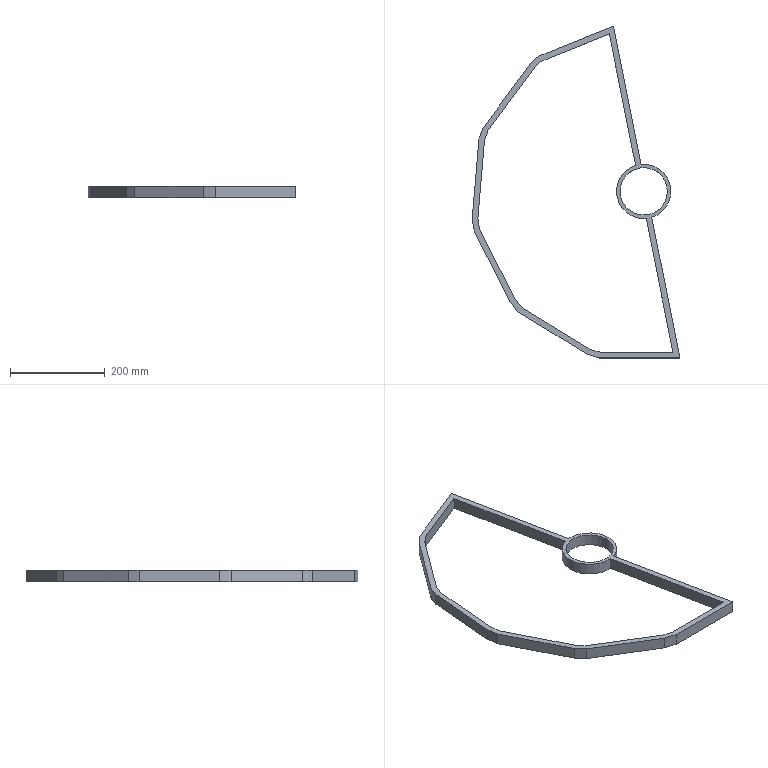Part | SolidWorks | features ICE 2, Extrusion 1 | 1 solid | 33 faces | box 439.055 x 701.743 x 25 mm | volume 573866 mm3 | plane 28 | cylinder 5 | commonest cylinder face diameters 115 x3 100 x2
STEP:
#1=CARTESIAN_POINT('',(25.649,-54.903,-12.5));
#2=VERTEX_POINT('',#1);
#3=CARTESIAN_POINT('',(66.063,0.,-12.5));
#4=VERTEX_POINT('',#3);
#5=CARTESIAN_POINT('',(8.563,0.,-12.5));
#6=DIRECTION('',(0.,0.,1.));
#7=DIRECTION('',(1.,0.,0.));
#8=AXIS2_PLACEMENT_3D('',#5,#6,#7);
#9=CIRCLE('',#8,57.5);
#10=EDGE_CURVE('',#2,#4,#9,.T.);
#11=ORIENTED_EDGE('',*,*,#10,.T.);
#12=CARTESIAN_POINT('',(66.063,0.,12.5));
#13=VERTEX_POINT('',#12);
#14=CARTESIAN_POINT('',(66.063,0.,-12.5));
#15=DIRECTION('',(0.,0.,1.));
#16=VECTOR('',#15,1000.);
#17=LINE('',#14,#16);
#18=EDGE_CURVE('',#4,#13,#17,.T.);
#19=ORIENTED_EDGE('',*,*,#18,.T.);
#20=CARTESIAN_POINT('',(25.649,-54.903,12.5));
#21=VERTEX_POINT('',#20);
#22=CARTESIAN_POINT('',(8.563,0.,12.5));
#23=DIRECTION('',(0.,0.,1.));
#24=DIRECTION('',(1.,0.,0.));
#25=AXIS2_PLACEMENT_3D('',#22,#23,#24);
#26=CIRCLE('',#25,57.5);
#27=EDGE_CURVE('',#21,#13,#26,.T.);
#28=ORIENTED_EDGE('',*,*,#27,.F.);
#29=CARTESIAN_POINT('',(25.649,-54.903,-12.5));
#30=DIRECTION('',(0.,0.,1.));
#31=VECTOR('',#30,1000.);
#32=LINE('',#29,#31);
#33=EDGE_CURVE('',#2,#21,#32,.T.);
#34=ORIENTED_EDGE('',*,*,#33,.F.);
#35=EDGE_LOOP('',(#11,#19,#28,#34));
#36=FACE_OUTER_BOUND('',#35,.T.);
#37=CARTESIAN_POINT('',(8.563,0.,-12.5));
#38=DIRECTION('',(0.,0.,1.));
#39=DIRECTION('',(1.,0.,0.));
#40=AXIS2_PLACEMENT_3D('',#37,#38,#39);
#41=CYLINDRICAL_SURFACE('',#40,57.5);
#42=ADVANCED_FACE('',(#36),#41,.T.);
#43=CARTESIAN_POINT('',(58.563,0.,-12.5));
#44=VERTEX_POINT('',#43);
#45=CARTESIAN_POINT('',(-41.437,0.,-12.5));
#46=VERTEX_POINT('',#45);
#47=CARTESIAN_POINT('',(8.563,0.,-12.5));
#48=DIRECTION('',(0.,0.,-1.));
#49=DIRECTION('',(-1.,0.,0.));
#50=AXIS2_PLACEMENT_3D('',#47,#48,#49);
#51=CIRCLE('',#50,50.);
#52=EDGE_CURVE('',#44,#46,#51,.T.);
#53=ORIENTED_EDGE('',*,*,#52,.T.);
#54=CARTESIAN_POINT('',(-41.437,0.,12.5));
#55=VERTEX_POINT('',#54);
#56=CARTESIAN_POINT('',(-41.437,0.,-27.5));
#57=DIRECTION('',(0.,0.,1.));
#58=VECTOR('',#57,1000.);
#59=LINE('',#56,#58);
#60=EDGE_CURVE('',#46,#55,#59,.T.);
#61=ORIENTED_EDGE('',*,*,#60,.T.);
#62=CARTESIAN_POINT('',(58.563,0.,12.5));
#63=VERTEX_POINT('',#62);
#64=CARTESIAN_POINT('',(8.563,0.,12.5));
#65=DIRECTION('',(0.,0.,1.));
#66=DIRECTION('',(1.,0.,0.));
#67=AXIS2_PLACEMENT_3D('',#64,#65,#66);
#68=CIRCLE('',#67,50.);
#69=EDGE_CURVE('',#55,#63,#68,.T.);
#70=ORIENTED_EDGE('',*,*,#69,.T.);
#71=CARTESIAN_POINT('',(58.563,0.,-27.5));
#72=DIRECTION('',(0.,0.,1.));
#73=VECTOR('',#72,1000.);
#74=LINE('',#71,#73);
#75=EDGE_CURVE('',#44,#63,#74,.T.);
#76=ORIENTED_EDGE('',*,*,#75,.F.);
#77=EDGE_LOOP('',(#53,#61,#70,#76));
#78=FACE_OUTER_BOUND('',#77,.T.);
#79=CARTESIAN_POINT('',(8.563,0.,-27.5));
#80=DIRECTION('',(0.,0.,1.));
#81=DIRECTION('',(1.,0.,0.));
#82=AXIS2_PLACEMENT_3D('',#79,#80,#81);
#83=CYLINDRICAL_SURFACE('',#82,50.);
#84=ADVANCED_FACE('',(#78),#83,.F.);
#85=CARTESIAN_POINT('',(85.,-352.,-12.5));
#86=VERTEX_POINT('',#85);
#87=CARTESIAN_POINT('',(85.,-352.,-12.5));
#88=DIRECTION('',(-0.1959,0.9806,0.));
#89=VECTOR('',#88,1000.);
#90=LINE('',#87,#89);
#91=EDGE_CURVE('',#86,#2,#90,.T.);
#92=ORIENTED_EDGE('',*,*,#91,.T.);
#93=ORIENTED_EDGE('',*,*,#33,.T.);
#94=CARTESIAN_POINT('',(85.,-352.,12.5));
#95=VERTEX_POINT('',#94);
#96=CARTESIAN_POINT('',(85.,-352.,12.5));
#97=DIRECTION('',(-0.1959,0.9806,0.));
#98=VECTOR('',#97,1000.);
#99=LINE('',#96,#98);
#100=EDGE_CURVE('',#95,#21,#99,.T.);
#101=ORIENTED_EDGE('',*,*,#100,.F.);
#102=CARTESIAN_POINT('',(85.,-352.,12.5));
#103=DIRECTION('',(0.,0.,-1.));
#104=VECTOR('',#103,1000.);
#105=LINE('',#102,#104);
#106=EDGE_CURVE('',#95,#86,#105,.T.);
#107=ORIENTED_EDGE('',*,*,#106,.T.);
#108=EDGE_LOOP('',(#92,#93,#101,#107));
#109=FACE_OUTER_BOUND('',#108,.T.);
#110=CARTESIAN_POINT('',(85.,-352.,12.5));
#111=DIRECTION('',(-0.9806,-0.1959,0.));
#112=DIRECTION('',(0.1959,-0.9806,0.));
#113=AXIS2_PLACEMENT_3D('',#110,#111,#112);
#114=PLANE('',#113);
#115=ADVANCED_FACE('',(#109),#114,.F.);
#116=CARTESIAN_POINT('',(13.882,-57.253,-12.5));
#117=VERTEX_POINT('',#116);
#118=CARTESIAN_POINT('',(13.882,-57.253,12.5));
#119=VERTEX_POINT('',#118);
#120=CARTESIAN_POINT('',(13.882,-57.253,-12.5));
#121=DIRECTION('',(0.,0.,1.));
#122=VECTOR('',#121,1000.);
#123=LINE('',#120,#122);
#124=EDGE_CURVE('',#117,#119,#123,.T.);
#125=ORIENTED_EDGE('',*,*,#124,.F.);
#126=CARTESIAN_POINT('',(70.366,-340.,-12.5));
#127=VERTEX_POINT('',#126);
#128=CARTESIAN_POINT('',(70.366,-340.,-12.5));
#129=DIRECTION('',(-0.1959,0.9806,0.));
#130=VECTOR('',#129,1000.);
#131=LINE('',#128,#130);
#132=EDGE_CURVE('',#127,#117,#131,.T.);
#133=ORIENTED_EDGE('',*,*,#132,.F.);
#134=CARTESIAN_POINT('',(70.366,-340.,12.5));
#135=VERTEX_POINT('',#134);
#136=CARTESIAN_POINT('',(70.366,-340.,12.5));
#137=DIRECTION('',(0.,0.,-1.));
#138=VECTOR('',#137,1000.);
#139=LINE('',#136,#138);
#140=EDGE_CURVE('',#135,#127,#139,.T.);
#141=ORIENTED_EDGE('',*,*,#140,.F.);
#142=CARTESIAN_POINT('',(70.366,-340.,12.5));
#143=DIRECTION('',(-0.1959,0.9806,0.));
#144=VECTOR('',#143,1000.);
#145=LINE('',#142,#144);
#146=EDGE_CURVE('',#135,#119,#145,.T.);
#147=ORIENTED_EDGE('',*,*,#146,.T.);
#148=EDGE_LOOP('',(#125,#133,#141,#147));
#149=FACE_OUTER_BOUND('',#148,.T.);
#150=CARTESIAN_POINT('',(70.366,-340.,12.5));
#151=DIRECTION('',(-0.9806,-0.1959,0.));
#152=DIRECTION('',(0.1959,-0.9806,0.));
#153=AXIS2_PLACEMENT_3D('',#150,#151,#152);
#154=PLANE('',#153);
#155=ADVANCED_FACE('',(#149),#154,.T.);
#156=CARTESIAN_POINT('',(8.563,0.,12.5));
#157=DIRECTION('',(0.,0.,1.));
#158=DIRECTION('',(1.,0.,0.));
#159=AXIS2_PLACEMENT_3D('',#156,#157,#158);
#160=CIRCLE('',#159,50.);
#161=EDGE_CURVE('',#63,#55,#160,.T.);
#162=ORIENTED_EDGE('',*,*,#161,.F.);
#163=ORIENTED_EDGE('',*,*,#69,.F.);
#164=EDGE_LOOP('',(#162,#163));
#165=FACE_BOUND('',#164,.T.);
#166=ORIENTED_EDGE('',*,*,#100,.T.);
#167=ORIENTED_EDGE('',*,*,#27,.T.);
#168=CARTESIAN_POINT('',(3.244,57.253,12.5));
#169=VERTEX_POINT('',#168);
#170=CARTESIAN_POINT('',(8.563,0.,12.5));
#171=DIRECTION('',(0.,0.,1.));
#172=DIRECTION('',(1.,0.,0.));
#173=AXIS2_PLACEMENT_3D('',#170,#171,#172);
#174=CIRCLE('',#173,57.5);
#175=EDGE_CURVE('',#13,#169,#174,.T.);
#176=ORIENTED_EDGE('',*,*,#175,.T.);
#177=CARTESIAN_POINT('',(-55.186,349.743,12.5));
#178=VERTEX_POINT('',#177);
#179=CARTESIAN_POINT('',(85.,-352.,12.5));
#180=DIRECTION('',(-0.1959,0.9806,0.));
#181=VECTOR('',#180,1000.);
#182=LINE('',#179,#181);
#183=EDGE_CURVE('',#169,#178,#182,.T.);
#184=ORIENTED_EDGE('',*,*,#183,.T.);
#185=CARTESIAN_POINT('',(-212.825,286.053,12.5));
#186=VERTEX_POINT('',#185);
#187=CARTESIAN_POINT('',(-55.186,349.743,12.5));
#188=DIRECTION('',(-0.9272,-0.3746,0.));
#189=VECTOR('',#188,1000.);
#190=LINE('',#187,#189);
#191=EDGE_CURVE('',#178,#186,#190,.T.);
#192=ORIENTED_EDGE('',*,*,#191,.T.);
#193=CARTESIAN_POINT('',(-230.576,270.461,12.5));
#194=VERTEX_POINT('',#193);
#195=CARTESIAN_POINT('',(-212.825,286.053,12.5));
#196=DIRECTION('',(-0.7513,-0.6599,0.));
#197=VECTOR('',#196,1000.);
#198=LINE('',#195,#197);
#199=EDGE_CURVE('',#186,#194,#198,.T.);
#200=ORIENTED_EDGE('',*,*,#199,.T.);
#201=CARTESIAN_POINT('',(-331.464,133.619,12.5));
#202=VERTEX_POINT('',#201);
#203=CARTESIAN_POINT('',(-230.576,270.461,12.5));
#204=DIRECTION('',(-0.5934,-0.8049,0.));
#205=VECTOR('',#204,1000.);
#206=LINE('',#203,#205);
#207=EDGE_CURVE('',#194,#202,#206,.T.);
#208=ORIENTED_EDGE('',*,*,#207,.T.);
#209=CARTESIAN_POINT('',(-339.829,110.705,12.5));
#210=VERTEX_POINT('',#209);
#211=CARTESIAN_POINT('',(-331.464,133.619,12.5));
#212=DIRECTION('',(-0.3429,-0.9394,0.));
#213=VECTOR('',#212,1000.);
#214=LINE('',#211,#213);
#215=EDGE_CURVE('',#202,#210,#214,.T.);
#216=ORIENTED_EDGE('',*,*,#215,.T.);
#217=CARTESIAN_POINT('',(-354.055,-58.706,12.5));
#218=VERTEX_POINT('',#217);
#219=CARTESIAN_POINT('',(-339.829,110.705,12.5));
#220=DIRECTION('',(-0.08368,-0.9965,0.));
#221=VECTOR('',#220,1000.);
#222=LINE('',#219,#221);
#223=EDGE_CURVE('',#210,#218,#222,.T.);
#224=ORIENTED_EDGE('',*,*,#223,.T.);
#225=CARTESIAN_POINT('',(-349.658,-83.74,12.5));
#226=VERTEX_POINT('',#225);
#227=CARTESIAN_POINT('',(-354.055,-58.706,12.5));
#228=DIRECTION('',(0.173,-0.9849,0.));
#229=VECTOR('',#228,1000.);
#230=LINE('',#227,#229);
#231=EDGE_CURVE('',#218,#226,#230,.T.);
#232=ORIENTED_EDGE('',*,*,#231,.T.);
#233=CARTESIAN_POINT('',(-273.007,-235.482,12.5));
#234=VERTEX_POINT('',#233);
#235=CARTESIAN_POINT('',(-349.658,-83.74,12.5));
#236=DIRECTION('',(0.4509,-0.8926,0.));
#237=VECTOR('',#236,1000.);
#238=LINE('',#235,#237);
#239=EDGE_CURVE('',#226,#234,#238,.T.);
#240=ORIENTED_EDGE('',*,*,#239,.T.);
#241=CARTESIAN_POINT('',(-255.616,-255.285,12.5));
#242=VERTEX_POINT('',#241);
#243=CARTESIAN_POINT('',(-273.007,-235.482,12.5));
#244=DIRECTION('',(0.6599,-0.7514,0.));
#245=VECTOR('',#244,1000.);
#246=LINE('',#243,#245);
#247=EDGE_CURVE('',#234,#242,#246,.T.);
#248=ORIENTED_EDGE('',*,*,#247,.T.);
#249=CARTESIAN_POINT('',(-110.822,-344.363,12.5));
#250=VERTEX_POINT('',#249);
#251=CARTESIAN_POINT('',(-255.616,-255.285,12.5));
#252=DIRECTION('',(0.8517,-0.524,0.));
#253=VECTOR('',#252,1000.);
#254=LINE('',#251,#253);
#255=EDGE_CURVE('',#242,#250,#254,.T.);
#256=ORIENTED_EDGE('',*,*,#255,.T.);
#257=CARTESIAN_POINT('',(-85.,-352.,12.5));
#258=VERTEX_POINT('',#257);
#259=CARTESIAN_POINT('',(-110.822,-344.363,12.5));
#260=DIRECTION('',(0.9589,-0.2836,0.));
#261=VECTOR('',#260,1000.);
#262=LINE('',#259,#261);
#263=EDGE_CURVE('',#250,#258,#262,.T.);
#264=ORIENTED_EDGE('',*,*,#263,.T.);
#265=CARTESIAN_POINT('',(-10.,-352.,12.5));
#266=DIRECTION('',(1.,0.,0.));
#267=VECTOR('',#266,1000.);
#268=LINE('',#265,#267);
#269=EDGE_CURVE('',#258,#95,#268,.T.);
#270=ORIENTED_EDGE('',*,*,#269,.T.);
#271=EDGE_LOOP('',(#166,#167,#176,#184,#192,#200,#208,#216,#224,#232,#240,#248,#256,#264,#270));
#272=FACE_OUTER_BOUND('',#271,.T.);
#273=CARTESIAN_POINT('',(-8.523,54.903,12.5));
#274=VERTEX_POINT('',#273);
#275=CARTESIAN_POINT('',(-64.117,333.193,12.5));
#276=VERTEX_POINT('',#275);
#277=CARTESIAN_POINT('',(70.366,-340.,12.5));
#278=DIRECTION('',(-0.1959,0.9806,0.));
#279=VECTOR('',#278,1000.);
#280=LINE('',#277,#279);
#281=EDGE_CURVE('',#274,#276,#280,.T.);
#282=ORIENTED_EDGE('',*,*,#281,.F.);
#283=CARTESIAN_POINT('',(8.563,0.,12.5));
#284=DIRECTION('',(0.,0.,1.));
#285=DIRECTION('',(1.,0.,0.));
#286=AXIS2_PLACEMENT_3D('',#283,#284,#285);
#287=CIRCLE('',#286,57.5);
#288=EDGE_CURVE('',#274,#119,#287,.T.);
#289=ORIENTED_EDGE('',*,*,#288,.T.);
#290=ORIENTED_EDGE('',*,*,#146,.F.);
#291=CARTESIAN_POINT('',(-83.263,-340.,12.5));
#292=VERTEX_POINT('',#291);
#293=CARTESIAN_POINT('',(-83.263,-340.,12.5));
#294=DIRECTION('',(1.,0.,0.));
#295=VECTOR('',#294,1000.);
#296=LINE('',#293,#295);
#297=EDGE_CURVE('',#292,#135,#296,.T.);
#298=ORIENTED_EDGE('',*,*,#297,.F.);
#299=CARTESIAN_POINT('',(-105.891,-333.308,12.5));
#300=VERTEX_POINT('',#299);
#301=CARTESIAN_POINT('',(-105.891,-333.308,12.5));
#302=DIRECTION('',(0.9589,-0.2836,0.));
#303=VECTOR('',#302,1000.);
#304=LINE('',#301,#303);
#305=EDGE_CURVE('',#300,#292,#304,.T.);
#306=ORIENTED_EDGE('',*,*,#305,.F.);
#307=CARTESIAN_POINT('',(-247.791,-246.011,12.5));
#308=VERTEX_POINT('',#307);
#309=CARTESIAN_POINT('',(-247.791,-246.011,12.5));
#310=DIRECTION('',(0.8517,-0.524,0.));
#311=VECTOR('',#310,1000.);
#312=LINE('',#309,#311);
#313=EDGE_CURVE('',#308,#300,#312,.T.);
#314=ORIENTED_EDGE('',*,*,#313,.F.);
#315=CARTESIAN_POINT('',(-262.984,-228.71,12.5));
#316=VERTEX_POINT('',#315);
#317=CARTESIAN_POINT('',(-262.984,-228.71,12.5));
#318=DIRECTION('',(0.6599,-0.7514,0.));
#319=VECTOR('',#318,1000.);
#320=LINE('',#317,#319);
#321=EDGE_CURVE('',#316,#308,#320,.T.);
#322=ORIENTED_EDGE('',*,*,#321,.F.);
#323=CARTESIAN_POINT('',(-338.146,-79.915,12.5));
#324=VERTEX_POINT('',#323);
#325=CARTESIAN_POINT('',(-338.146,-79.915,12.5));
#326=DIRECTION('',(0.4509,-0.8926,0.));
#327=VECTOR('',#326,1000.);
#328=LINE('',#325,#327);
#329=EDGE_CURVE('',#324,#316,#328,.T.);
#330=ORIENTED_EDGE('',*,*,#329,.F.);
#331=CARTESIAN_POINT('',(-341.967,-58.161,12.5));
#332=VERTEX_POINT('',#331);
#333=CARTESIAN_POINT('',(-341.967,-58.161,12.5));
#334=DIRECTION('',(0.173,-0.9849,0.));
#335=VECTOR('',#334,1000.);
#336=LINE('',#333,#335);
#337=EDGE_CURVE('',#332,#324,#336,.T.);
#338=ORIENTED_EDGE('',*,*,#337,.F.);
#339=CARTESIAN_POINT('',(-328.005,108.1,12.5));
#340=VERTEX_POINT('',#339);
#341=CARTESIAN_POINT('',(-328.005,108.1,12.5));
#342=DIRECTION('',(-0.08368,-0.9965,0.));
#343=VECTOR('',#342,1000.);
#344=LINE('',#341,#343);
#345=EDGE_CURVE('',#340,#332,#344,.T.);
#346=ORIENTED_EDGE('',*,*,#345,.F.);
#347=CARTESIAN_POINT('',(-320.783,127.885,12.5));
#348=VERTEX_POINT('',#347);
#349=CARTESIAN_POINT('',(-320.783,127.885,12.5));
#350=DIRECTION('',(-0.3429,-0.9394,0.));
#351=VECTOR('',#350,1000.);
#352=LINE('',#349,#351);
#353=EDGE_CURVE('',#348,#340,#352,.T.);
#354=ORIENTED_EDGE('',*,*,#353,.F.);
#355=CARTESIAN_POINT('',(-221.685,262.298,12.5));
#356=VERTEX_POINT('',#355);
#357=CARTESIAN_POINT('',(-221.685,262.298,12.5));
#358=DIRECTION('',(-0.5934,-0.8049,0.));
#359=VECTOR('',#358,1000.);
#360=LINE('',#357,#359);
#361=EDGE_CURVE('',#356,#348,#360,.T.);
#362=ORIENTED_EDGE('',*,*,#361,.F.);
#363=CARTESIAN_POINT('',(-206.438,275.691,12.5));
#364=VERTEX_POINT('',#363);
#365=CARTESIAN_POINT('',(-206.438,275.691,12.5));
#366=DIRECTION('',(-0.7513,-0.6599,0.));
#367=VECTOR('',#366,1000.);
#368=LINE('',#365,#367);
#369=EDGE_CURVE('',#364,#356,#368,.T.);
#370=ORIENTED_EDGE('',*,*,#369,.F.);
#371=CARTESIAN_POINT('',(-120.237,310.518,12.5));
#372=DIRECTION('',(-0.9272,-0.3746,0.));
#373=VECTOR('',#372,1000.);
#374=LINE('',#371,#373);
#375=EDGE_CURVE('',#276,#364,#374,.T.);
#376=ORIENTED_EDGE('',*,*,#375,.F.);
#377=EDGE_LOOP('',(#282,#289,#290,#298,#306,#314,#322,#330,#338,#346,#354,#362,#370,#376));
#378=FACE_BOUND('',#377,.T.);
#379=CARTESIAN_POINT('',(0.,0.,12.5));
#380=DIRECTION('',(0.,0.,-1.));
#381=DIRECTION('',(-1.,0.,0.));
#382=AXIS2_PLACEMENT_3D('',#379,#380,#381);
#383=PLANE('',#382);
#384=ADVANCED_FACE('',(#165,#272,#378),#383,.F.);
#385=ORIENTED_EDGE('',*,*,#52,.F.);
#386=CARTESIAN_POINT('',(8.563,0.,-12.5));
#387=DIRECTION('',(0.,0.,-1.));
#388=DIRECTION('',(-1.,0.,0.));
#389=AXIS2_PLACEMENT_3D('',#386,#387,#388);
#390=CIRCLE('',#389,50.);
#391=EDGE_CURVE('',#46,#44,#390,.T.);
#392=ORIENTED_EDGE('',*,*,#391,.F.);
#393=EDGE_LOOP('',(#385,#392));
#394=FACE_BOUND('',#393,.T.);
#395=ORIENTED_EDGE('',*,*,#10,.F.);
#396=ORIENTED_EDGE('',*,*,#91,.F.);
#397=CARTESIAN_POINT('',(-85.,-352.,-12.5));
#398=VERTEX_POINT('',#397);
#399=CARTESIAN_POINT('',(-85.,-352.,-12.5));
#400=DIRECTION('',(1.,0.,0.));
#401=VECTOR('',#400,1000.);
#402=LINE('',#399,#401);
#403=EDGE_CURVE('',#398,#86,#402,.T.);
#404=ORIENTED_EDGE('',*,*,#403,.F.);
#405=CARTESIAN_POINT('',(-110.822,-344.363,-12.5));
#406=VERTEX_POINT('',#405);
#407=CARTESIAN_POINT('',(-110.822,-344.363,-12.5));
#408=DIRECTION('',(0.9589,-0.2836,0.));
#409=VECTOR('',#408,1000.);
#410=LINE('',#407,#409);
#411=EDGE_CURVE('',#406,#398,#410,.T.);
#412=ORIENTED_EDGE('',*,*,#411,.F.);
#413=CARTESIAN_POINT('',(-255.616,-255.285,-12.5));
#414=VERTEX_POINT('',#413);
#415=CARTESIAN_POINT('',(-174.702,-305.064,-12.5));
#416=DIRECTION('',(0.8517,-0.524,0.));
#417=VECTOR('',#416,1000.);
#418=LINE('',#415,#417);
#419=EDGE_CURVE('',#414,#406,#418,.T.);
#420=ORIENTED_EDGE('',*,*,#419,.F.);
#421=CARTESIAN_POINT('',(-273.007,-235.482,-12.5));
#422=VERTEX_POINT('',#421);
#423=CARTESIAN_POINT('',(-273.007,-235.482,-12.5));
#424=DIRECTION('',(0.6599,-0.7514,0.));
#425=VECTOR('',#424,1000.);
#426=LINE('',#423,#425);
#427=EDGE_CURVE('',#422,#414,#426,.T.);
#428=ORIENTED_EDGE('',*,*,#427,.F.);
#429=CARTESIAN_POINT('',(-349.658,-83.74,-12.5));
#430=VERTEX_POINT('',#429);
#431=CARTESIAN_POINT('',(-306.824,-168.537,-12.5));
#432=DIRECTION('',(0.4509,-0.8926,0.));
#433=VECTOR('',#432,1000.);
#434=LINE('',#431,#433);
#435=EDGE_CURVE('',#430,#422,#434,.T.);
#436=ORIENTED_EDGE('',*,*,#435,.F.);
#437=CARTESIAN_POINT('',(-354.055,-58.706,-12.5));
#438=VERTEX_POINT('',#437);
#439=CARTESIAN_POINT('',(-354.055,-58.706,-12.5));
#440=DIRECTION('',(0.173,-0.9849,0.));
#441=VECTOR('',#440,1000.);
#442=LINE('',#439,#441);
#443=EDGE_CURVE('',#438,#430,#442,.T.);
#444=ORIENTED_EDGE('',*,*,#443,.F.);
#445=CARTESIAN_POINT('',(-339.829,110.705,-12.5));
#446=VERTEX_POINT('',#445);
#447=CARTESIAN_POINT('',(-347.779,16.034,-12.5));
#448=DIRECTION('',(-0.08368,-0.9965,0.));
#449=VECTOR('',#448,1000.);
#450=LINE('',#447,#449);
#451=EDGE_CURVE('',#446,#438,#450,.T.);
#452=ORIENTED_EDGE('',*,*,#451,.F.);
#453=CARTESIAN_POINT('',(-331.464,133.619,-12.5));
#454=VERTEX_POINT('',#453);
#455=CARTESIAN_POINT('',(-331.464,133.619,-12.5));
#456=DIRECTION('',(-0.3429,-0.9394,0.));
#457=VECTOR('',#456,1000.);
#458=LINE('',#455,#457);
#459=EDGE_CURVE('',#454,#446,#458,.T.);
#460=ORIENTED_EDGE('',*,*,#459,.F.);
#461=CARTESIAN_POINT('',(-230.576,270.461,-12.5));
#462=VERTEX_POINT('',#461);
#463=CARTESIAN_POINT('',(-286.955,193.99,-12.5));
#464=DIRECTION('',(-0.5934,-0.8049,0.));
#465=VECTOR('',#464,1000.);
#466=LINE('',#463,#465);
#467=EDGE_CURVE('',#462,#454,#466,.T.);
#468=ORIENTED_EDGE('',*,*,#467,.F.);
#469=CARTESIAN_POINT('',(-212.825,286.053,-12.5));
#470=VERTEX_POINT('',#469);
#471=CARTESIAN_POINT('',(-212.825,286.053,-12.5));
#472=DIRECTION('',(-0.7513,-0.6599,0.));
#473=VECTOR('',#472,1000.);
#474=LINE('',#471,#473);
#475=EDGE_CURVE('',#470,#462,#474,.T.);
#476=ORIENTED_EDGE('',*,*,#475,.F.);
#477=CARTESIAN_POINT('',(-55.186,349.743,-12.5));
#478=VERTEX_POINT('',#477);
#479=CARTESIAN_POINT('',(-143.278,314.152,-12.5));
#480=DIRECTION('',(-0.9272,-0.3746,0.));
#481=VECTOR('',#480,1000.);
#482=LINE('',#479,#481);
#483=EDGE_CURVE('',#478,#470,#482,.T.);
#484=ORIENTED_EDGE('',*,*,#483,.F.);
#485=CARTESIAN_POINT('',(3.244,57.253,-12.5));
#486=VERTEX_POINT('',#485);
#487=CARTESIAN_POINT('',(85.,-352.,-12.5));
#488=DIRECTION('',(-0.1959,0.9806,0.));
#489=VECTOR('',#488,1000.);
#490=LINE('',#487,#489);
#491=EDGE_CURVE('',#486,#478,#490,.T.);
#492=ORIENTED_EDGE('',*,*,#491,.F.);
#493=CARTESIAN_POINT('',(8.563,0.,-12.5));
#494=DIRECTION('',(0.,0.,1.));
#495=DIRECTION('',(1.,0.,0.));
#496=AXIS2_PLACEMENT_3D('',#493,#494,#495);
#497=CIRCLE('',#496,57.5);
#498=EDGE_CURVE('',#4,#486,#497,.T.);
#499=ORIENTED_EDGE('',*,*,#498,.F.);
#500=EDGE_LOOP('',(#395,#396,#404,#412,#420,#428,#436,#444,#452,#460,#468,#476,#484,#492,#499));
#501=FACE_OUTER_BOUND('',#500,.T.);
#502=ORIENTED_EDGE('',*,*,#132,.T.);
#503=CARTESIAN_POINT('',(-8.523,54.903,-12.5));
#504=VERTEX_POINT('',#503);
#505=CARTESIAN_POINT('',(8.563,0.,-12.5));
#506=DIRECTION('',(0.,0.,1.));
#507=DIRECTION('',(1.,0.,0.));
#508=AXIS2_PLACEMENT_3D('',#505,#506,#507);
#509=CIRCLE('',#508,57.5);
#510=EDGE_CURVE('',#504,#117,#509,.T.);
#511=ORIENTED_EDGE('',*,*,#510,.F.);
#512=CARTESIAN_POINT('',(-64.117,333.193,-12.5));
#513=VERTEX_POINT('',#512);
#514=CARTESIAN_POINT('',(70.366,-340.,-12.5));
#515=DIRECTION('',(-0.1959,0.9806,0.));
#516=VECTOR('',#515,1000.);
#517=LINE('',#514,#516);
#518=EDGE_CURVE('',#504,#513,#517,.T.);
#519=ORIENTED_EDGE('',*,*,#518,.T.);
#520=CARTESIAN_POINT('',(-206.438,275.691,-12.5));
#521=VERTEX_POINT('',#520);
#522=CARTESIAN_POINT('',(-64.117,333.193,-12.5));
#523=DIRECTION('',(-0.9272,-0.3746,0.));
#524=VECTOR('',#523,1000.);
#525=LINE('',#522,#524);
#526=EDGE_CURVE('',#513,#521,#525,.T.);
#527=ORIENTED_EDGE('',*,*,#526,.T.);
#528=CARTESIAN_POINT('',(-221.685,262.298,-12.5));
#529=VERTEX_POINT('',#528);
#530=CARTESIAN_POINT('',(-206.438,275.691,-12.5));
#531=DIRECTION('',(-0.7513,-0.6599,0.));
#532=VECTOR('',#531,1000.);
#533=LINE('',#530,#532);
#534=EDGE_CURVE('',#521,#529,#533,.T.);
#535=ORIENTED_EDGE('',*,*,#534,.T.);
#536=CARTESIAN_POINT('',(-320.783,127.885,-12.5));
#537=VERTEX_POINT('',#536);
#538=CARTESIAN_POINT('',(-277.296,186.869,-12.5));
#539=DIRECTION('',(-0.5934,-0.8049,0.));
#540=VECTOR('',#539,1000.);
#541=LINE('',#538,#540);
#542=EDGE_CURVE('',#529,#537,#541,.T.);
#543=ORIENTED_EDGE('',*,*,#542,.T.);
#544=CARTESIAN_POINT('',(-328.005,108.1,-12.5));
#545=VERTEX_POINT('',#544);
#546=CARTESIAN_POINT('',(-320.783,127.885,-12.5));
#547=DIRECTION('',(-0.3429,-0.9394,0.));
#548=VECTOR('',#547,1000.);
#549=LINE('',#546,#548);
#550=EDGE_CURVE('',#537,#545,#549,.T.);
#551=ORIENTED_EDGE('',*,*,#550,.T.);
#552=CARTESIAN_POINT('',(-341.967,-58.161,-12.5));
#553=VERTEX_POINT('',#552);
#554=CARTESIAN_POINT('',(-335.821,15.03,-12.5));
#555=DIRECTION('',(-0.08368,-0.9965,0.));
#556=VECTOR('',#555,1000.);
#557=LINE('',#554,#556);
#558=EDGE_CURVE('',#545,#553,#557,.T.);
#559=ORIENTED_EDGE('',*,*,#558,.T.);
#560=CARTESIAN_POINT('',(-338.146,-79.915,-12.5));
#561=VERTEX_POINT('',#560);
#562=CARTESIAN_POINT('',(-341.967,-58.161,-12.5));
#563=DIRECTION('',(0.173,-0.9849,0.));
#564=VECTOR('',#563,1000.);
#565=LINE('',#562,#564);
#566=EDGE_CURVE('',#553,#561,#565,.T.);
#567=ORIENTED_EDGE('',*,*,#566,.T.);
#568=CARTESIAN_POINT('',(-262.984,-228.71,-12.5));
#569=VERTEX_POINT('',#568);
#570=CARTESIAN_POINT('',(-296.113,-163.126,-12.5));
#571=DIRECTION('',(0.4509,-0.8926,0.));
#572=VECTOR('',#571,1000.);
#573=LINE('',#570,#572);
#574=EDGE_CURVE('',#561,#569,#573,.T.);
#575=ORIENTED_EDGE('',*,*,#574,.T.);
#576=CARTESIAN_POINT('',(-247.791,-246.011,-12.5));
#577=VERTEX_POINT('',#576);
#578=CARTESIAN_POINT('',(-262.984,-228.71,-12.5));
#579=DIRECTION('',(0.6599,-0.7514,0.));
#580=VECTOR('',#579,1000.);
#581=LINE('',#578,#580);
#582=EDGE_CURVE('',#569,#577,#581,.T.);
#583=ORIENTED_EDGE('',*,*,#582,.T.);
#584=CARTESIAN_POINT('',(-105.891,-333.308,-12.5));
#585=VERTEX_POINT('',#584);
#586=CARTESIAN_POINT('',(-168.414,-294.844,-12.5));
#587=DIRECTION('',(0.8517,-0.524,0.));
#588=VECTOR('',#587,1000.);
#589=LINE('',#586,#588);
#590=EDGE_CURVE('',#577,#585,#589,.T.);
#591=ORIENTED_EDGE('',*,*,#590,.T.);
#592=CARTESIAN_POINT('',(-83.263,-340.,-12.5));
#593=VERTEX_POINT('',#592);
#594=CARTESIAN_POINT('',(-105.891,-333.308,-12.5));
#595=DIRECTION('',(0.9589,-0.2836,0.));
#596=VECTOR('',#595,1000.);
#597=LINE('',#594,#596);
#598=EDGE_CURVE('',#585,#593,#597,.T.);
#599=ORIENTED_EDGE('',*,*,#598,.T.);
#600=CARTESIAN_POINT('',(10.,-340.,-12.5));
#601=DIRECTION('',(1.,0.,0.));
#602=VECTOR('',#601,1000.);
#603=LINE('',#600,#602);
#604=EDGE_CURVE('',#593,#127,#603,.T.);
#605=ORIENTED_EDGE('',*,*,#604,.T.);
#606=EDGE_LOOP('',(#502,#511,#519,#527,#535,#543,#551,#559,#567,#575,#583,#591,#599,#605));
#607=FACE_BOUND('',#606,.T.);
#608=CARTESIAN_POINT('',(0.,0.,-12.5));
#609=DIRECTION('',(0.,0.,-1.));
#610=DIRECTION('',(-1.,0.,0.));
#611=AXIS2_PLACEMENT_3D('',#608,#609,#610);
#612=PLANE('',#611);
#613=ADVANCED_FACE('',(#394,#501,#607),#612,.T.);
#614=ORIENTED_EDGE('',*,*,#183,.F.);
#615=CARTESIAN_POINT('',(3.244,57.253,-12.5));
#616=DIRECTION('',(0.,0.,-1.));
#617=VECTOR('',#616,1000.);
#618=LINE('',#615,#617);
#619=EDGE_CURVE('',#169,#486,#618,.T.);
#620=ORIENTED_EDGE('',*,*,#619,.T.);
#621=ORIENTED_EDGE('',*,*,#491,.T.);
#622=CARTESIAN_POINT('',(-55.186,349.743,12.5));
#623=DIRECTION('',(0.,0.,-1.));
#624=VECTOR('',#623,1000.);
#625=LINE('',#622,#624);
#626=EDGE_CURVE('',#178,#478,#625,.T.);
#627=ORIENTED_EDGE('',*,*,#626,.F.);
#628=EDGE_LOOP('',(#614,#620,#621,#627));
#629=FACE_OUTER_BOUND('',#628,.T.);
#630=CARTESIAN_POINT('',(85.,-352.,12.5));
#631=DIRECTION('',(-0.9806,-0.1959,0.));
#632=DIRECTION('',(0.1959,-0.9806,0.));
#633=AXIS2_PLACEMENT_3D('',#630,#631,#632);
#634=PLANE('',#633);
#635=ADVANCED_FACE('',(#629),#634,.F.);
#636=ORIENTED_EDGE('',*,*,#483,.T.);
#637=CARTESIAN_POINT('',(-212.825,286.053,12.5));
#638=DIRECTION('',(0.,0.,-1.));
#639=VECTOR('',#638,1000.);
#640=LINE('',#637,#639);
#641=EDGE_CURVE('',#186,#470,#640,.T.);
#642=ORIENTED_EDGE('',*,*,#641,.F.);
#643=ORIENTED_EDGE('',*,*,#191,.F.);
#644=ORIENTED_EDGE('',*,*,#626,.T.);
#645=EDGE_LOOP('',(#636,#642,#643,#644));
#646=FACE_OUTER_BOUND('',#645,.T.);
#647=CARTESIAN_POINT('',(-143.278,314.152,12.5));
#648=DIRECTION('',(0.3746,-0.9272,0.));
#649=DIRECTION('',(0.9272,0.3746,0.));
#650=AXIS2_PLACEMENT_3D('',#647,#648,#649);
#651=PLANE('',#650);
#652=ADVANCED_FACE('',(#646),#651,.F.);
#653=ORIENTED_EDGE('',*,*,#475,.T.);
#654=CARTESIAN_POINT('',(-230.576,270.461,12.5));
#655=DIRECTION('',(0.,0.,-1.));
#656=VECTOR('',#655,1000.);
#657=LINE('',#654,#656);
#658=EDGE_CURVE('',#194,#462,#657,.T.);
#659=ORIENTED_EDGE('',*,*,#658,.F.);
#660=ORIENTED_EDGE('',*,*,#199,.F.);
#661=ORIENTED_EDGE('',*,*,#641,.T.);
#662=EDGE_LOOP('',(#653,#659,#660,#661));
#663=FACE_OUTER_BOUND('',#662,.T.);
#664=CARTESIAN_POINT('',(-212.825,286.053,12.5));
#665=DIRECTION('',(0.6599,-0.7513,0.));
#666=DIRECTION('',(0.7513,0.6599,0.));
#667=AXIS2_PLACEMENT_3D('',#664,#665,#666);
#668=PLANE('',#667);
#669=ADVANCED_FACE('',(#663),#668,.F.);
#670=ORIENTED_EDGE('',*,*,#467,.T.);
#671=CARTESIAN_POINT('',(-331.464,133.619,12.5));
#672=DIRECTION('',(0.,0.,-1.));
#673=VECTOR('',#672,1000.);
#674=LINE('',#671,#673);
#675=EDGE_CURVE('',#202,#454,#674,.T.);
#676=ORIENTED_EDGE('',*,*,#675,.F.);
#677=ORIENTED_EDGE('',*,*,#207,.F.);
#678=ORIENTED_EDGE('',*,*,#658,.T.);
#679=EDGE_LOOP('',(#670,#676,#677,#678));
#680=FACE_OUTER_BOUND('',#679,.T.);
#681=CARTESIAN_POINT('',(-286.955,193.99,12.5));
#682=DIRECTION('',(0.8049,-0.5934,0.));
#683=DIRECTION('',(0.5934,0.8049,0.));
#684=AXIS2_PLACEMENT_3D('',#681,#682,#683);
#685=PLANE('',#684);
#686=ADVANCED_FACE('',(#680),#685,.F.);
#687=ORIENTED_EDGE('',*,*,#459,.T.);
#688=CARTESIAN_POINT('',(-339.829,110.705,12.5));
#689=DIRECTION('',(0.,0.,-1.));
#690=VECTOR('',#689,1000.);
#691=LINE('',#688,#690);
#692=EDGE_CURVE('',#210,#446,#691,.T.);
#693=ORIENTED_EDGE('',*,*,#692,.F.);
#694=ORIENTED_EDGE('',*,*,#215,.F.);
#695=ORIENTED_EDGE('',*,*,#675,.T.);
#696=EDGE_LOOP('',(#687,#693,#694,#695));
#697=FACE_OUTER_BOUND('',#696,.T.);
#698=CARTESIAN_POINT('',(-331.464,133.619,12.5));
#699=DIRECTION('',(0.9394,-0.3429,0.));
#700=DIRECTION('',(0.3429,0.9394,0.));
#701=AXIS2_PLACEMENT_3D('',#698,#699,#700);
#702=PLANE('',#701);
#703=ADVANCED_FACE('',(#697),#702,.F.);
#704=ORIENTED_EDGE('',*,*,#451,.T.);
#705=CARTESIAN_POINT('',(-354.055,-58.706,12.5));
#706=DIRECTION('',(0.,0.,-1.));
#707=VECTOR('',#706,1000.);
#708=LINE('',#705,#707);
#709=EDGE_CURVE('',#218,#438,#708,.T.);
#710=ORIENTED_EDGE('',*,*,#709,.F.);
#711=ORIENTED_EDGE('',*,*,#223,.F.);
#712=ORIENTED_EDGE('',*,*,#692,.T.);
#713=EDGE_LOOP('',(#704,#710,#711,#712));
#714=FACE_OUTER_BOUND('',#713,.T.);
#715=CARTESIAN_POINT('',(-347.779,16.034,12.5));
#716=DIRECTION('',(0.9965,-0.08368,0.));
#717=DIRECTION('',(0.08368,0.9965,0.));
#718=AXIS2_PLACEMENT_3D('',#715,#716,#717);
#719=PLANE('',#718);
#720=ADVANCED_FACE('',(#714),#719,.F.);
#721=ORIENTED_EDGE('',*,*,#443,.T.);
#722=CARTESIAN_POINT('',(-349.658,-83.74,12.5));
#723=DIRECTION('',(0.,0.,-1.));
#724=VECTOR('',#723,1000.);
#725=LINE('',#722,#724);
#726=EDGE_CURVE('',#226,#430,#725,.T.);
#727=ORIENTED_EDGE('',*,*,#726,.F.);
#728=ORIENTED_EDGE('',*,*,#231,.F.);
#729=ORIENTED_EDGE('',*,*,#709,.T.);
#730=EDGE_LOOP('',(#721,#727,#728,#729));
#731=FACE_OUTER_BOUND('',#730,.T.);
#732=CARTESIAN_POINT('',(-354.055,-58.706,12.5));
#733=DIRECTION('',(0.9849,0.173,0.));
#734=DIRECTION('',(-0.173,0.9849,0.));
#735=AXIS2_PLACEMENT_3D('',#732,#733,#734);
#736=PLANE('',#735);
#737=ADVANCED_FACE('',(#731),#736,.F.);
#738=ORIENTED_EDGE('',*,*,#435,.T.);
#739=CARTESIAN_POINT('',(-273.007,-235.482,12.5));
#740=DIRECTION('',(0.,0.,-1.));
#741=VECTOR('',#740,1000.);
#742=LINE('',#739,#741);
#743=EDGE_CURVE('',#234,#422,#742,.T.);
#744=ORIENTED_EDGE('',*,*,#743,.F.);
#745=ORIENTED_EDGE('',*,*,#239,.F.);
#746=ORIENTED_EDGE('',*,*,#726,.T.);
#747=EDGE_LOOP('',(#738,#744,#745,#746));
#748=FACE_OUTER_BOUND('',#747,.T.);
#749=CARTESIAN_POINT('',(-306.824,-168.537,12.5));
#750=DIRECTION('',(0.8926,0.4509,0.));
#751=DIRECTION('',(-0.4509,0.8926,0.));
#752=AXIS2_PLACEMENT_3D('',#749,#750,#751);
#753=PLANE('',#752);
#754=ADVANCED_FACE('',(#748),#753,.F.);
#755=ORIENTED_EDGE('',*,*,#427,.T.);
#756=CARTESIAN_POINT('',(-255.616,-255.285,12.5));
#757=DIRECTION('',(0.,0.,-1.));
#758=VECTOR('',#757,1000.);
#759=LINE('',#756,#758);
#760=EDGE_CURVE('',#242,#414,#759,.T.);
#761=ORIENTED_EDGE('',*,*,#760,.F.);
#762=ORIENTED_EDGE('',*,*,#247,.F.);
#763=ORIENTED_EDGE('',*,*,#743,.T.);
#764=EDGE_LOOP('',(#755,#761,#762,#763));
#765=FACE_OUTER_BOUND('',#764,.T.);
#766=CARTESIAN_POINT('',(-273.007,-235.482,12.5));
#767=DIRECTION('',(0.7514,0.6599,0.));
#768=DIRECTION('',(-0.6599,0.7514,0.));
#769=AXIS2_PLACEMENT_3D('',#766,#767,#768);
#770=PLANE('',#769);
#771=ADVANCED_FACE('',(#765),#770,.F.);
#772=ORIENTED_EDGE('',*,*,#419,.T.);
#773=CARTESIAN_POINT('',(-110.822,-344.363,12.5));
#774=DIRECTION('',(0.,0.,-1.));
#775=VECTOR('',#774,1000.);
#776=LINE('',#773,#775);
#777=EDGE_CURVE('',#250,#406,#776,.T.);
#778=ORIENTED_EDGE('',*,*,#777,.F.);
#779=ORIENTED_EDGE('',*,*,#255,.F.);
#780=ORIENTED_EDGE('',*,*,#760,.T.);
#781=EDGE_LOOP('',(#772,#778,#779,#780));
#782=FACE_OUTER_BOUND('',#781,.T.);
#783=CARTESIAN_POINT('',(-174.702,-305.064,12.5));
#784=DIRECTION('',(0.524,0.8517,0.));
#785=DIRECTION('',(-0.8517,0.524,0.));
#786=AXIS2_PLACEMENT_3D('',#783,#784,#785);
#787=PLANE('',#786);
#788=ADVANCED_FACE('',(#782),#787,.F.);
#789=ORIENTED_EDGE('',*,*,#411,.T.);
#790=CARTESIAN_POINT('',(-85.,-352.,12.5));
#791=DIRECTION('',(0.,0.,-1.));
#792=VECTOR('',#791,1000.);
#793=LINE('',#790,#792);
#794=EDGE_CURVE('',#258,#398,#793,.T.);
#795=ORIENTED_EDGE('',*,*,#794,.F.);
#796=ORIENTED_EDGE('',*,*,#263,.F.);
#797=ORIENTED_EDGE('',*,*,#777,.T.);
#798=EDGE_LOOP('',(#789,#795,#796,#797));
#799=FACE_OUTER_BOUND('',#798,.T.);
#800=CARTESIAN_POINT('',(-110.822,-344.363,12.5));
#801=DIRECTION('',(0.2836,0.9589,0.));
#802=DIRECTION('',(-0.9589,0.2836,0.));
#803=AXIS2_PLACEMENT_3D('',#800,#801,#802);
#804=PLANE('',#803);
#805=ADVANCED_FACE('',(#799),#804,.F.);
#806=ORIENTED_EDGE('',*,*,#403,.T.);
#807=ORIENTED_EDGE('',*,*,#106,.F.);
#808=ORIENTED_EDGE('',*,*,#269,.F.);
#809=ORIENTED_EDGE('',*,*,#794,.T.);
#810=EDGE_LOOP('',(#806,#807,#808,#809));
#811=FACE_OUTER_BOUND('',#810,.T.);
#812=CARTESIAN_POINT('',(-85.,-352.,12.5));
#813=DIRECTION('',(0.,1.,0.));
#814=DIRECTION('',(0.,0.,1.));
#815=AXIS2_PLACEMENT_3D('',#812,#813,#814);
#816=PLANE('',#815);
#817=ADVANCED_FACE('',(#811),#816,.F.);
#818=ORIENTED_EDGE('',*,*,#534,.F.);
#819=CARTESIAN_POINT('',(-206.438,275.691,12.5));
#820=DIRECTION('',(0.,0.,-1.));
#821=VECTOR('',#820,1000.);
#822=LINE('',#819,#821);
#823=EDGE_CURVE('',#364,#521,#822,.T.);
#824=ORIENTED_EDGE('',*,*,#823,.F.);
#825=ORIENTED_EDGE('',*,*,#369,.T.);
#826=CARTESIAN_POINT('',(-221.685,262.298,12.5));
#827=DIRECTION('',(0.,0.,-1.));
#828=VECTOR('',#827,1000.);
#829=LINE('',#826,#828);
#830=EDGE_CURVE('',#356,#529,#829,.T.);
#831=ORIENTED_EDGE('',*,*,#830,.T.);
#832=EDGE_LOOP('',(#818,#824,#825,#831));
#833=FACE_OUTER_BOUND('',#832,.T.);
#834=CARTESIAN_POINT('',(-206.438,275.691,12.5));
#835=DIRECTION('',(0.6599,-0.7513,0.));
#836=DIRECTION('',(0.7513,0.6599,0.));
#837=AXIS2_PLACEMENT_3D('',#834,#835,#836);
#838=PLANE('',#837);
#839=ADVANCED_FACE('',(#833),#838,.T.);
#840=ORIENTED_EDGE('',*,*,#542,.F.);
#841=ORIENTED_EDGE('',*,*,#830,.F.);
#842=ORIENTED_EDGE('',*,*,#361,.T.);
#843=CARTESIAN_POINT('',(-320.783,127.885,12.5));
#844=DIRECTION('',(0.,0.,-1.));
#845=VECTOR('',#844,1000.);
#846=LINE('',#843,#845);
#847=EDGE_CURVE('',#348,#537,#846,.T.);
#848=ORIENTED_EDGE('',*,*,#847,.T.);
#849=EDGE_LOOP('',(#840,#841,#842,#848));
#850=FACE_OUTER_BOUND('',#849,.T.);
#851=CARTESIAN_POINT('',(-277.296,186.869,12.5));
#852=DIRECTION('',(0.8049,-0.5934,0.));
#853=DIRECTION('',(0.5934,0.8049,0.));
#854=AXIS2_PLACEMENT_3D('',#851,#852,#853);
#855=PLANE('',#854);
#856=ADVANCED_FACE('',(#850),#855,.T.);
#857=ORIENTED_EDGE('',*,*,#550,.F.);
#858=ORIENTED_EDGE('',*,*,#847,.F.);
#859=ORIENTED_EDGE('',*,*,#353,.T.);
#860=CARTESIAN_POINT('',(-328.005,108.1,12.5));
#861=DIRECTION('',(0.,0.,-1.));
#862=VECTOR('',#861,1000.);
#863=LINE('',#860,#862);
#864=EDGE_CURVE('',#340,#545,#863,.T.);
#865=ORIENTED_EDGE('',*,*,#864,.T.);
#866=EDGE_LOOP('',(#857,#858,#859,#865));
#867=FACE_OUTER_BOUND('',#866,.T.);
#868=CARTESIAN_POINT('',(-320.783,127.885,12.5));
#869=DIRECTION('',(0.9394,-0.3429,0.));
#870=DIRECTION('',(0.3429,0.9394,0.));
#871=AXIS2_PLACEMENT_3D('',#868,#869,#870);
#872=PLANE('',#871);
#873=ADVANCED_FACE('',(#867),#872,.T.);
#874=ORIENTED_EDGE('',*,*,#558,.F.);
#875=ORIENTED_EDGE('',*,*,#864,.F.);
#876=ORIENTED_EDGE('',*,*,#345,.T.);
#877=CARTESIAN_POINT('',(-341.967,-58.161,12.5));
#878=DIRECTION('',(0.,0.,-1.));
#879=VECTOR('',#878,1000.);
#880=LINE('',#877,#879);
#881=EDGE_CURVE('',#332,#553,#880,.T.);
#882=ORIENTED_EDGE('',*,*,#881,.T.);
#883=EDGE_LOOP('',(#874,#875,#876,#882));
#884=FACE_OUTER_BOUND('',#883,.T.);
#885=CARTESIAN_POINT('',(-335.821,15.03,12.5));
#886=DIRECTION('',(0.9965,-0.08368,0.));
#887=DIRECTION('',(0.08368,0.9965,0.));
#888=AXIS2_PLACEMENT_3D('',#885,#886,#887);
#889=PLANE('',#888);
#890=ADVANCED_FACE('',(#884),#889,.T.);
#891=ORIENTED_EDGE('',*,*,#566,.F.);
#892=ORIENTED_EDGE('',*,*,#881,.F.);
#893=ORIENTED_EDGE('',*,*,#337,.T.);
#894=CARTESIAN_POINT('',(-338.146,-79.915,12.5));
#895=DIRECTION('',(0.,0.,-1.));
#896=VECTOR('',#895,1000.);
#897=LINE('',#894,#896);
#898=EDGE_CURVE('',#324,#561,#897,.T.);
#899=ORIENTED_EDGE('',*,*,#898,.T.);
#900=EDGE_LOOP('',(#891,#892,#893,#899));
#901=FACE_OUTER_BOUND('',#900,.T.);
#902=CARTESIAN_POINT('',(-341.967,-58.161,12.5));
#903=DIRECTION('',(0.9849,0.173,0.));
#904=DIRECTION('',(-0.173,0.9849,0.));
#905=AXIS2_PLACEMENT_3D('',#902,#903,#904);
#906=PLANE('',#905);
#907=ADVANCED_FACE('',(#901),#906,.T.);
#908=ORIENTED_EDGE('',*,*,#574,.F.);
#909=ORIENTED_EDGE('',*,*,#898,.F.);
#910=ORIENTED_EDGE('',*,*,#329,.T.);
#911=CARTESIAN_POINT('',(-262.984,-228.71,12.5));
#912=DIRECTION('',(0.,0.,-1.));
#913=VECTOR('',#912,1000.);
#914=LINE('',#911,#913);
#915=EDGE_CURVE('',#316,#569,#914,.T.);
#916=ORIENTED_EDGE('',*,*,#915,.T.);
#917=EDGE_LOOP('',(#908,#909,#910,#916));
#918=FACE_OUTER_BOUND('',#917,.T.);
#919=CARTESIAN_POINT('',(-296.113,-163.126,12.5));
#920=DIRECTION('',(0.8926,0.4509,0.));
#921=DIRECTION('',(-0.4509,0.8926,0.));
#922=AXIS2_PLACEMENT_3D('',#919,#920,#921);
#923=PLANE('',#922);
#924=ADVANCED_FACE('',(#918),#923,.T.);
#925=ORIENTED_EDGE('',*,*,#582,.F.);
#926=ORIENTED_EDGE('',*,*,#915,.F.);
#927=ORIENTED_EDGE('',*,*,#321,.T.);
#928=CARTESIAN_POINT('',(-247.791,-246.011,12.5));
#929=DIRECTION('',(0.,0.,-1.));
#930=VECTOR('',#929,1000.);
#931=LINE('',#928,#930);
#932=EDGE_CURVE('',#308,#577,#931,.T.);
#933=ORIENTED_EDGE('',*,*,#932,.T.);
#934=EDGE_LOOP('',(#925,#926,#927,#933));
#935=FACE_OUTER_BOUND('',#934,.T.);
#936=CARTESIAN_POINT('',(-262.984,-228.71,12.5));
#937=DIRECTION('',(0.7514,0.6599,0.));
#938=DIRECTION('',(-0.6599,0.7514,0.));
#939=AXIS2_PLACEMENT_3D('',#936,#937,#938);
#940=PLANE('',#939);
#941=ADVANCED_FACE('',(#935),#940,.T.);
#942=ORIENTED_EDGE('',*,*,#590,.F.);
#943=ORIENTED_EDGE('',*,*,#932,.F.);
#944=ORIENTED_EDGE('',*,*,#313,.T.);
#945=CARTESIAN_POINT('',(-105.891,-333.308,12.5));
#946=DIRECTION('',(0.,0.,-1.));
#947=VECTOR('',#946,1000.);
#948=LINE('',#945,#947);
#949=EDGE_CURVE('',#300,#585,#948,.T.);
#950=ORIENTED_EDGE('',*,*,#949,.T.);
#951=EDGE_LOOP('',(#942,#943,#944,#950));
#952=FACE_OUTER_BOUND('',#951,.T.);
#953=CARTESIAN_POINT('',(-168.414,-294.844,12.5));
#954=DIRECTION('',(0.524,0.8517,0.));
#955=DIRECTION('',(-0.8517,0.524,0.));
#956=AXIS2_PLACEMENT_3D('',#953,#954,#955);
#957=PLANE('',#956);
#958=ADVANCED_FACE('',(#952),#957,.T.);
#959=ORIENTED_EDGE('',*,*,#598,.F.);
#960=ORIENTED_EDGE('',*,*,#949,.F.);
#961=ORIENTED_EDGE('',*,*,#305,.T.);
#962=CARTESIAN_POINT('',(-83.263,-340.,12.5));
#963=DIRECTION('',(0.,0.,-1.));
#964=VECTOR('',#963,1000.);
#965=LINE('',#962,#964);
#966=EDGE_CURVE('',#292,#593,#965,.T.);
#967=ORIENTED_EDGE('',*,*,#966,.T.);
#968=EDGE_LOOP('',(#959,#960,#961,#967));
#969=FACE_OUTER_BOUND('',#968,.T.);
#970=CARTESIAN_POINT('',(-105.891,-333.308,12.5));
#971=DIRECTION('',(0.2836,0.9589,0.));
#972=DIRECTION('',(-0.9589,0.2836,0.));
#973=AXIS2_PLACEMENT_3D('',#970,#971,#972);
#974=PLANE('',#973);
#975=ADVANCED_FACE('',(#969),#974,.T.);
#976=ORIENTED_EDGE('',*,*,#604,.F.);
#977=ORIENTED_EDGE('',*,*,#966,.F.);
#978=ORIENTED_EDGE('',*,*,#297,.T.);
#979=ORIENTED_EDGE('',*,*,#140,.T.);
#980=EDGE_LOOP('',(#976,#977,#978,#979));
#981=FACE_OUTER_BOUND('',#980,.T.);
#982=CARTESIAN_POINT('',(10.,-340.,12.5));
#983=DIRECTION('',(0.,1.,0.));
#984=DIRECTION('',(0.,0.,1.));
#985=AXIS2_PLACEMENT_3D('',#982,#983,#984);
#986=PLANE('',#985);
#987=ADVANCED_FACE('',(#981),#986,.T.);
#988=CARTESIAN_POINT('',(-8.523,54.903,-12.5));
#989=DIRECTION('',(0.,0.,-1.));
#990=VECTOR('',#989,1000.);
#991=LINE('',#988,#990);
#992=EDGE_CURVE('',#274,#504,#991,.T.);
#993=ORIENTED_EDGE('',*,*,#992,.F.);
#994=ORIENTED_EDGE('',*,*,#281,.T.);
#995=CARTESIAN_POINT('',(-64.117,333.193,12.5));
#996=DIRECTION('',(0.,0.,-1.));
#997=VECTOR('',#996,1000.);
#998=LINE('',#995,#997);
#999=EDGE_CURVE('',#276,#513,#998,.T.);
#1000=ORIENTED_EDGE('',*,*,#999,.T.);
#1001=ORIENTED_EDGE('',*,*,#518,.F.);
#1002=EDGE_LOOP('',(#993,#994,#1000,#1001));
#1003=FACE_OUTER_BOUND('',#1002,.T.);
#1004=CARTESIAN_POINT('',(70.366,-340.,12.5));
#1005=DIRECTION('',(-0.9806,-0.1959,0.));
#1006=DIRECTION('',(0.1959,-0.9806,0.));
#1007=AXIS2_PLACEMENT_3D('',#1004,#1005,#1006);
#1008=PLANE('',#1007);
#1009=ADVANCED_FACE('',(#1003),#1008,.T.);
#1010=ORIENTED_EDGE('',*,*,#526,.F.);
#1011=ORIENTED_EDGE('',*,*,#999,.F.);
#1012=ORIENTED_EDGE('',*,*,#375,.T.);
#1013=ORIENTED_EDGE('',*,*,#823,.T.);
#1014=EDGE_LOOP('',(#1010,#1011,#1012,#1013));
#1015=FACE_OUTER_BOUND('',#1014,.T.);
#1016=CARTESIAN_POINT('',(-64.117,333.193,12.5));
#1017=DIRECTION('',(0.3746,-0.9272,0.));
#1018=DIRECTION('',(0.9272,0.3746,0.));
#1019=AXIS2_PLACEMENT_3D('',#1016,#1017,#1018);
#1020=PLANE('',#1019);
#1021=ADVANCED_FACE('',(#1015),#1020,.T.);
#1022=ORIENTED_EDGE('',*,*,#60,.F.);
#1023=ORIENTED_EDGE('',*,*,#391,.T.);
#1024=ORIENTED_EDGE('',*,*,#75,.T.);
#1025=ORIENTED_EDGE('',*,*,#161,.T.);
#1026=EDGE_LOOP('',(#1022,#1023,#1024,#1025));
#1027=FACE_OUTER_BOUND('',#1026,.T.);
#1028=CARTESIAN_POINT('',(8.563,0.,-27.5));
#1029=DIRECTION('',(0.,0.,1.));
#1030=DIRECTION('',(1.,0.,0.));
#1031=AXIS2_PLACEMENT_3D('',#1028,#1029,#1030);
#1032=CYLINDRICAL_SURFACE('',#1031,50.);
#1033=ADVANCED_FACE('',(#1027),#1032,.F.);
#1034=ORIENTED_EDGE('',*,*,#510,.T.);
#1035=ORIENTED_EDGE('',*,*,#124,.T.);
#1036=ORIENTED_EDGE('',*,*,#288,.F.);
#1037=ORIENTED_EDGE('',*,*,#992,.T.);
#1038=EDGE_LOOP('',(#1034,#1035,#1036,#1037));
#1039=FACE_OUTER_BOUND('',#1038,.T.);
#1040=CARTESIAN_POINT('',(8.563,0.,-12.5));
#1041=DIRECTION('',(0.,0.,1.));
#1042=DIRECTION('',(1.,0.,0.));
#1043=AXIS2_PLACEMENT_3D('',#1040,#1041,#1042);
#1044=CYLINDRICAL_SURFACE('',#1043,57.5);
#1045=ADVANCED_FACE('',(#1039),#1044,.T.);
#1046=ORIENTED_EDGE('',*,*,#18,.F.);
#1047=ORIENTED_EDGE('',*,*,#498,.T.);
#1048=ORIENTED_EDGE('',*,*,#619,.F.);
#1049=ORIENTED_EDGE('',*,*,#175,.F.);
#1050=EDGE_LOOP('',(#1046,#1047,#1048,#1049));
#1051=FACE_OUTER_BOUND('',#1050,.T.);
#1052=CARTESIAN_POINT('',(8.563,0.,-12.5));
#1053=DIRECTION('',(0.,0.,1.));
#1054=DIRECTION('',(1.,0.,0.));
#1055=AXIS2_PLACEMENT_3D('',#1052,#1053,#1054);
#1056=CYLINDRICAL_SURFACE('',#1055,57.5);
#1057=ADVANCED_FACE('',(#1051),#1056,.T.);
#1058=CLOSED_SHELL('',(#42,#84,#115,#155,#384,#613,#635,#652,#669,#686,#703,#720,#737,#754,#771,#788,#805,#817,#839,#856,#873,#890,#907,#924,#941,#958,#975,#987,#1009,#1021,#1033,#1045,#1057));
#1059=MANIFOLD_SOLID_BREP('',#1058);
#1060=CARTESIAN_POINT('',(0.,0.,0.));
#1061=DIRECTION('',(0.,0.,1.));
#1062=DIRECTION('',(1.,0.,0.));
#1063=AXIS2_PLACEMENT_3D('',#1060,#1061,#1062);
#1064=(LENGTH_UNIT()NAMED_UNIT(*)SI_UNIT(.MILLI.,.METRE.));
#1065=UNCERTAINTY_MEASURE_WITH_UNIT(LENGTH_MEASURE(0.00001),#1064,'','');
#1066=(NAMED_UNIT(*)PLANE_ANGLE_UNIT()SI_UNIT($,.RADIAN.));
#1067=(NAMED_UNIT(*)SI_UNIT($,.STERADIAN.)SOLID_ANGLE_UNIT());
#1068=(GEOMETRIC_REPRESENTATION_CONTEXT(3)GLOBAL_UNCERTAINTY_ASSIGNED_CONTEXT((#1065))GLOBAL_UNIT_ASSIGNED_CONTEXT((#1064,#1066,#1067))REPRESENTATION_CONTEXT('',''));
#1069=ADVANCED_BREP_SHAPE_REPRESENTATION('',(#1059,#1063),#1068);